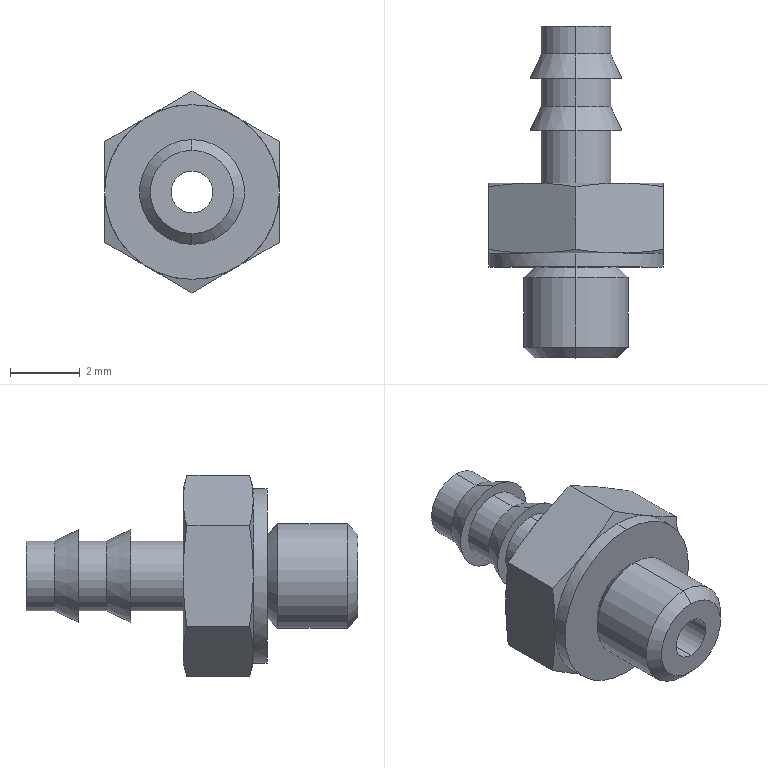Part | STEP file | M-3AU-3 | 1 solid | 44 faces | box 5 x 9.5 x 5.774 mm | volume 73.564 mm3 | cone 20 | cylinder 12 | plane 12 | commonest cylinder face diameters 2 x6 1.2 x2 3 x2 5 x2
STEP:
#1=CARTESIAN_POINT('',(0.,6.9,0.6));
#2=VERTEX_POINT('',#1);
#3=CARTESIAN_POINT('',(0.,6.9,-0.6));
#4=VERTEX_POINT('',#3);
#5=CARTESIAN_POINT('',(0.,6.9,0.));
#6=DIRECTION('',(0.,-1.,0.));
#7=DIRECTION('',(0.,0.,-1.));
#8=AXIS2_PLACEMENT_3D('',#5,#6,#7);
#9=CIRCLE('',#8,0.6);
#10=EDGE_CURVE('',#2,#4,#9,.T.);
#11=ORIENTED_EDGE('',*,*,#10,.F.);
#12=CARTESIAN_POINT('',(0.,-2.6,0.6));
#13=VERTEX_POINT('',#12);
#14=CARTESIAN_POINT('',(0.,2.15,0.6));
#15=DIRECTION('',(0.,-1.,0.));
#16=VECTOR('',#15,1000.);
#17=LINE('',#14,#16);
#18=EDGE_CURVE('',#2,#13,#17,.T.);
#19=ORIENTED_EDGE('',*,*,#18,.T.);
#20=CARTESIAN_POINT('',(0.,-2.6,-0.6));
#21=VERTEX_POINT('',#20);
#22=CARTESIAN_POINT('',(0.,-2.6,0.));
#23=DIRECTION('',(0.,1.,0.));
#24=DIRECTION('',(0.,0.,-1.));
#25=AXIS2_PLACEMENT_3D('',#22,#23,#24);
#26=CIRCLE('',#25,0.6);
#27=EDGE_CURVE('',#21,#13,#26,.T.);
#28=ORIENTED_EDGE('',*,*,#27,.F.);
#29=CARTESIAN_POINT('',(0.,2.15,-0.6));
#30=DIRECTION('',(0.,-1.,0.));
#31=VECTOR('',#30,1000.);
#32=LINE('',#29,#31);
#33=EDGE_CURVE('',#4,#21,#32,.T.);
#34=ORIENTED_EDGE('',*,*,#33,.F.);
#35=EDGE_LOOP('',(#11,#19,#28,#34));
#36=FACE_OUTER_BOUND('',#35,.T.);
#37=CARTESIAN_POINT('',(0.,2.15,0.));
#38=DIRECTION('',(0.,-1.,0.));
#39=DIRECTION('',(0.,0.,-1.));
#40=AXIS2_PLACEMENT_3D('',#37,#38,#39);
#41=CYLINDRICAL_SURFACE('',#40,0.6);
#42=ADVANCED_FACE('',(#36),#41,.F.);
#43=CARTESIAN_POINT('',(0.,-2.6,-1.193));
#44=VERTEX_POINT('',#43);
#45=CARTESIAN_POINT('',(0.,-2.6,1.193));
#46=VERTEX_POINT('',#45);
#47=CARTESIAN_POINT('',(0.,-2.6,0.));
#48=DIRECTION('',(0.,-1.,0.));
#49=DIRECTION('',(0.,0.,1.));
#50=AXIS2_PLACEMENT_3D('',#47,#48,#49);
#51=CIRCLE('',#50,1.193);
#52=EDGE_CURVE('',#44,#46,#51,.T.);
#53=ORIENTED_EDGE('',*,*,#52,.F.);
#54=CARTESIAN_POINT('',(0.,-2.294,-1.5));
#55=VERTEX_POINT('',#54);
#56=CARTESIAN_POINT('',(0.,-2.294,-1.5));
#57=DIRECTION('',(0.,0.7071,-0.7071));
#58=VECTOR('',#57,1000.);
#59=LINE('',#56,#58);
#60=EDGE_CURVE('',#44,#55,#59,.T.);
#61=ORIENTED_EDGE('',*,*,#60,.T.);
#62=CARTESIAN_POINT('',(0.,-2.294,1.5));
#63=VERTEX_POINT('',#62);
#64=CARTESIAN_POINT('',(0.,-2.294,0.));
#65=DIRECTION('',(0.,-1.,0.));
#66=DIRECTION('',(1.,0.,0.));
#67=AXIS2_PLACEMENT_3D('',#64,#65,#66);
#68=CIRCLE('',#67,1.5);
#69=EDGE_CURVE('',#55,#63,#68,.T.);
#70=ORIENTED_EDGE('',*,*,#69,.T.);
#71=CARTESIAN_POINT('',(0.,-2.294,1.5));
#72=DIRECTION('',(0.,0.7071,0.7071));
#73=VECTOR('',#72,1000.);
#74=LINE('',#71,#73);
#75=EDGE_CURVE('',#46,#63,#74,.T.);
#76=ORIENTED_EDGE('',*,*,#75,.F.);
#77=EDGE_LOOP('',(#53,#61,#70,#76));
#78=FACE_OUTER_BOUND('',#77,.T.);
#79=CARTESIAN_POINT('',(0.,-2.294,0.));
#80=DIRECTION('',(0.,1.,0.));
#81=DIRECTION('',(0.,0.,1.));
#82=AXIS2_PLACEMENT_3D('',#79,#80,#81);
#83=CONICAL_SURFACE('',#82,1.5,0.7854);
#84=ADVANCED_FACE('',(#78),#83,.T.);
#85=CARTESIAN_POINT('',(0.,6.9,1.));
#86=VERTEX_POINT('',#85);
#87=CARTESIAN_POINT('',(0.,6.9,-1.));
#88=VERTEX_POINT('',#87);
#89=CARTESIAN_POINT('',(0.,6.9,0.));
#90=DIRECTION('',(0.,1.,0.));
#91=DIRECTION('',(0.,0.,-1.));
#92=AXIS2_PLACEMENT_3D('',#89,#90,#91);
#93=CIRCLE('',#92,1.);
#94=EDGE_CURVE('',#86,#88,#93,.T.);
#95=ORIENTED_EDGE('',*,*,#94,.F.);
#96=CARTESIAN_POINT('',(0.,6.1,1.));
#97=VERTEX_POINT('',#96);
#98=CARTESIAN_POINT('',(0.,6.5,1.));
#99=DIRECTION('',(0.,-1.,0.));
#100=VECTOR('',#99,1000.);
#101=LINE('',#98,#100);
#102=EDGE_CURVE('',#86,#97,#101,.T.);
#103=ORIENTED_EDGE('',*,*,#102,.T.);
#104=CARTESIAN_POINT('',(0.,6.1,-1.));
#105=VERTEX_POINT('',#104);
#106=CARTESIAN_POINT('',(0.,6.1,0.));
#107=DIRECTION('',(0.,1.,0.));
#108=DIRECTION('',(0.,0.,-1.));
#109=AXIS2_PLACEMENT_3D('',#106,#107,#108);
#110=CIRCLE('',#109,1.);
#111=EDGE_CURVE('',#97,#105,#110,.T.);
#112=ORIENTED_EDGE('',*,*,#111,.T.);
#113=CARTESIAN_POINT('',(0.,6.5,-1.));
#114=DIRECTION('',(0.,-1.,0.));
#115=VECTOR('',#114,1000.);
#116=LINE('',#113,#115);
#117=EDGE_CURVE('',#88,#105,#116,.T.);
#118=ORIENTED_EDGE('',*,*,#117,.F.);
#119=EDGE_LOOP('',(#95,#103,#112,#118));
#120=FACE_OUTER_BOUND('',#119,.T.);
#121=CARTESIAN_POINT('',(0.,6.5,0.));
#122=DIRECTION('',(0.,-1.,0.));
#123=DIRECTION('',(0.,0.,-1.));
#124=AXIS2_PLACEMENT_3D('',#121,#122,#123);
#125=CYLINDRICAL_SURFACE('',#124,1.);
#126=ADVANCED_FACE('',(#120),#125,.T.);
#127=CARTESIAN_POINT('',(0.,-0.3065,-1.5));
#128=VERTEX_POINT('',#127);
#129=CARTESIAN_POINT('',(0.,-0.3065,1.5));
#130=VERTEX_POINT('',#129);
#131=CARTESIAN_POINT('',(0.,-0.3065,0.));
#132=DIRECTION('',(0.,-1.,0.));
#133=DIRECTION('',(0.,0.,-1.));
#134=AXIS2_PLACEMENT_3D('',#131,#132,#133);
#135=CIRCLE('',#134,1.5);
#136=EDGE_CURVE('',#128,#130,#135,.T.);
#137=ORIENTED_EDGE('',*,*,#136,.T.);
#138=CARTESIAN_POINT('',(0.,-1.3,1.5));
#139=DIRECTION('',(0.,-1.,0.));
#140=VECTOR('',#139,1000.);
#141=LINE('',#138,#140);
#142=EDGE_CURVE('',#130,#63,#141,.T.);
#143=ORIENTED_EDGE('',*,*,#142,.T.);
#144=ORIENTED_EDGE('',*,*,#69,.F.);
#145=CARTESIAN_POINT('',(0.,-1.3,-1.5));
#146=DIRECTION('',(0.,-1.,0.));
#147=VECTOR('',#146,1000.);
#148=LINE('',#145,#147);
#149=EDGE_CURVE('',#128,#55,#148,.T.);
#150=ORIENTED_EDGE('',*,*,#149,.F.);
#151=EDGE_LOOP('',(#137,#143,#144,#150));
#152=FACE_OUTER_BOUND('',#151,.T.);
#153=CARTESIAN_POINT('',(0.,-1.3,0.));
#154=DIRECTION('',(0.,-1.,0.));
#155=DIRECTION('',(0.,0.,-1.));
#156=AXIS2_PLACEMENT_3D('',#153,#154,#155);
#157=CYLINDRICAL_SURFACE('',#156,1.5);
#158=ADVANCED_FACE('',(#152),#157,.T.);
#159=ORIENTED_EDGE('',*,*,#111,.F.);
#160=CARTESIAN_POINT('',(0.,5.4,1.326));
#161=VERTEX_POINT('',#160);
#162=CARTESIAN_POINT('',(0.,5.4,1.326));
#163=DIRECTION('',(0.,-0.9063,0.4226));
#164=VECTOR('',#163,1000.);
#165=LINE('',#162,#164);
#166=EDGE_CURVE('',#97,#161,#165,.T.);
#167=ORIENTED_EDGE('',*,*,#166,.T.);
#168=CARTESIAN_POINT('',(0.,5.4,-1.326));
#169=VERTEX_POINT('',#168);
#170=CARTESIAN_POINT('',(0.,5.4,0.));
#171=DIRECTION('',(0.,1.,0.));
#172=DIRECTION('',(0.,0.,-1.));
#173=AXIS2_PLACEMENT_3D('',#170,#171,#172);
#174=CIRCLE('',#173,1.326);
#175=EDGE_CURVE('',#161,#169,#174,.T.);
#176=ORIENTED_EDGE('',*,*,#175,.T.);
#177=CARTESIAN_POINT('',(0.,5.4,-1.326));
#178=DIRECTION('',(0.,-0.9063,-0.4226));
#179=VECTOR('',#178,1000.);
#180=LINE('',#177,#179);
#181=EDGE_CURVE('',#105,#169,#180,.T.);
#182=ORIENTED_EDGE('',*,*,#181,.F.);
#183=EDGE_LOOP('',(#159,#167,#176,#182));
#184=FACE_OUTER_BOUND('',#183,.T.);
#185=CARTESIAN_POINT('',(0.,5.4,0.));
#186=DIRECTION('',(0.,-1.,0.));
#187=DIRECTION('',(0.,0.,-1.));
#188=AXIS2_PLACEMENT_3D('',#185,#186,#187);
#189=CONICAL_SURFACE('',#188,1.326,0.4363);
#190=ADVANCED_FACE('',(#184),#189,.T.);
#191=CARTESIAN_POINT('',(0.,0.,-1.193));
#192=VERTEX_POINT('',#191);
#193=CARTESIAN_POINT('',(0.,0.,1.193));
#194=VERTEX_POINT('',#193);
#195=CARTESIAN_POINT('',(0.,0.,0.));
#196=DIRECTION('',(0.,-1.,0.));
#197=DIRECTION('',(0.,0.,-1.));
#198=AXIS2_PLACEMENT_3D('',#195,#196,#197);
#199=CIRCLE('',#198,1.193);
#200=EDGE_CURVE('',#192,#194,#199,.T.);
#201=ORIENTED_EDGE('',*,*,#200,.T.);
#202=CARTESIAN_POINT('',(0.,-0.3065,1.5));
#203=DIRECTION('',(0.,-0.7071,0.7071));
#204=VECTOR('',#203,1000.);
#205=LINE('',#202,#204);
#206=EDGE_CURVE('',#194,#130,#205,.T.);
#207=ORIENTED_EDGE('',*,*,#206,.T.);
#208=ORIENTED_EDGE('',*,*,#136,.F.);
#209=CARTESIAN_POINT('',(0.,-0.3065,-1.5));
#210=DIRECTION('',(0.,-0.7071,-0.7071));
#211=VECTOR('',#210,1000.);
#212=LINE('',#209,#211);
#213=EDGE_CURVE('',#192,#128,#212,.T.);
#214=ORIENTED_EDGE('',*,*,#213,.F.);
#215=EDGE_LOOP('',(#201,#207,#208,#214));
#216=FACE_OUTER_BOUND('',#215,.T.);
#217=CARTESIAN_POINT('',(0.,-0.3065,0.));
#218=DIRECTION('',(0.,-1.,0.));
#219=DIRECTION('',(0.,0.,-1.));
#220=AXIS2_PLACEMENT_3D('',#217,#218,#219);
#221=CONICAL_SURFACE('',#220,1.5,0.7854);
#222=ADVANCED_FACE('',(#216),#221,.T.);
#223=CARTESIAN_POINT('',(0.,5.4,1.));
#224=VERTEX_POINT('',#223);
#225=CARTESIAN_POINT('',(0.,5.4,-1.));
#226=VERTEX_POINT('',#225);
#227=CARTESIAN_POINT('',(0.,5.4,0.));
#228=DIRECTION('',(0.,1.,0.));
#229=DIRECTION('',(0.,0.,-1.));
#230=AXIS2_PLACEMENT_3D('',#227,#228,#229);
#231=CIRCLE('',#230,1.);
#232=EDGE_CURVE('',#224,#226,#231,.T.);
#233=ORIENTED_EDGE('',*,*,#232,.F.);
#234=CARTESIAN_POINT('',(0.,4.6,1.));
#235=VERTEX_POINT('',#234);
#236=CARTESIAN_POINT('',(0.,5.,1.));
#237=DIRECTION('',(0.,-1.,0.));
#238=VECTOR('',#237,1000.);
#239=LINE('',#236,#238);
#240=EDGE_CURVE('',#224,#235,#239,.T.);
#241=ORIENTED_EDGE('',*,*,#240,.T.);
#242=CARTESIAN_POINT('',(0.,4.6,-1.));
#243=VERTEX_POINT('',#242);
#244=CARTESIAN_POINT('',(0.,4.6,0.));
#245=DIRECTION('',(0.,1.,0.));
#246=DIRECTION('',(0.,0.,-1.));
#247=AXIS2_PLACEMENT_3D('',#244,#245,#246);
#248=CIRCLE('',#247,1.);
#249=EDGE_CURVE('',#235,#243,#248,.T.);
#250=ORIENTED_EDGE('',*,*,#249,.T.);
#251=CARTESIAN_POINT('',(0.,5.,-1.));
#252=DIRECTION('',(0.,-1.,0.));
#253=VECTOR('',#252,1000.);
#254=LINE('',#251,#253);
#255=EDGE_CURVE('',#226,#243,#254,.T.);
#256=ORIENTED_EDGE('',*,*,#255,.F.);
#257=EDGE_LOOP('',(#233,#241,#250,#256));
#258=FACE_OUTER_BOUND('',#257,.T.);
#259=CARTESIAN_POINT('',(0.,5.,0.));
#260=DIRECTION('',(0.,-1.,0.));
#261=DIRECTION('',(0.,0.,-1.));
#262=AXIS2_PLACEMENT_3D('',#259,#260,#261);
#263=CYLINDRICAL_SURFACE('',#262,1.);
#264=ADVANCED_FACE('',(#258),#263,.T.);
#265=CARTESIAN_POINT('',(1.25,0.4,2.165));
#266=VERTEX_POINT('',#265);
#267=CARTESIAN_POINT('',(0.,0.4,2.5));
#268=VERTEX_POINT('',#267);
#269=CARTESIAN_POINT('',(0.,0.4,0.));
#270=DIRECTION('',(0.,-1.,0.));
#271=DIRECTION('',(0.,0.,-1.));
#272=AXIS2_PLACEMENT_3D('',#269,#270,#271);
#273=CIRCLE('',#272,2.5);
#274=EDGE_CURVE('',#266,#268,#273,.T.);
#275=ORIENTED_EDGE('',*,*,#274,.T.);
#276=CARTESIAN_POINT('',(0.,0.,2.5));
#277=VERTEX_POINT('',#276);
#278=CARTESIAN_POINT('',(0.,0.2,2.5));
#279=DIRECTION('',(0.,-1.,0.));
#280=VECTOR('',#279,1000.);
#281=LINE('',#278,#280);
#282=EDGE_CURVE('',#268,#277,#281,.T.);
#283=ORIENTED_EDGE('',*,*,#282,.T.);
#284=CARTESIAN_POINT('',(0.,0.,-2.5));
#285=VERTEX_POINT('',#284);
#286=CARTESIAN_POINT('',(0.,0.,0.));
#287=DIRECTION('',(0.,-1.,0.));
#288=DIRECTION('',(0.,0.,-1.));
#289=AXIS2_PLACEMENT_3D('',#286,#287,#288);
#290=CIRCLE('',#289,2.5);
#291=EDGE_CURVE('',#285,#277,#290,.T.);
#292=ORIENTED_EDGE('',*,*,#291,.F.);
#293=CARTESIAN_POINT('',(0.,0.4,-2.5));
#294=VERTEX_POINT('',#293);
#295=CARTESIAN_POINT('',(0.,0.2,-2.5));
#296=DIRECTION('',(0.,-1.,0.));
#297=VECTOR('',#296,1000.);
#298=LINE('',#295,#297);
#299=EDGE_CURVE('',#294,#285,#298,.T.);
#300=ORIENTED_EDGE('',*,*,#299,.F.);
#301=CARTESIAN_POINT('',(1.25,0.4,-2.165));
#302=VERTEX_POINT('',#301);
#303=CARTESIAN_POINT('',(0.,0.4,0.));
#304=DIRECTION('',(0.,-1.,0.));
#305=DIRECTION('',(0.,0.,-1.));
#306=AXIS2_PLACEMENT_3D('',#303,#304,#305);
#307=CIRCLE('',#306,2.5);
#308=EDGE_CURVE('',#294,#302,#307,.T.);
#309=ORIENTED_EDGE('',*,*,#308,.T.);
#310=CARTESIAN_POINT('',(2.5,0.4,0.));
#311=VERTEX_POINT('',#310);
#312=CARTESIAN_POINT('',(0.,0.4,0.));
#313=DIRECTION('',(0.,-1.,0.));
#314=DIRECTION('',(0.,0.,-1.));
#315=AXIS2_PLACEMENT_3D('',#312,#313,#314);
#316=CIRCLE('',#315,2.5);
#317=EDGE_CURVE('',#302,#311,#316,.T.);
#318=ORIENTED_EDGE('',*,*,#317,.T.);
#319=CARTESIAN_POINT('',(0.,0.4,0.));
#320=DIRECTION('',(0.,-1.,0.));
#321=DIRECTION('',(0.,0.,-1.));
#322=AXIS2_PLACEMENT_3D('',#319,#320,#321);
#323=CIRCLE('',#322,2.5);
#324=EDGE_CURVE('',#311,#266,#323,.T.);
#325=ORIENTED_EDGE('',*,*,#324,.T.);
#326=EDGE_LOOP('',(#275,#283,#292,#300,#309,#318,#325));
#327=FACE_OUTER_BOUND('',#326,.T.);
#328=CARTESIAN_POINT('',(0.,0.2,0.));
#329=DIRECTION('',(0.,-1.,0.));
#330=DIRECTION('',(0.,0.,-1.));
#331=AXIS2_PLACEMENT_3D('',#328,#329,#330);
#332=CYLINDRICAL_SURFACE('',#331,2.5);
#333=ADVANCED_FACE('',(#327),#332,.T.);
#334=ORIENTED_EDGE('',*,*,#249,.F.);
#335=CARTESIAN_POINT('',(0.,3.9,1.326));
#336=VERTEX_POINT('',#335);
#337=CARTESIAN_POINT('',(0.,3.9,1.326));
#338=DIRECTION('',(0.,-0.9063,0.4226));
#339=VECTOR('',#338,1000.);
#340=LINE('',#337,#339);
#341=EDGE_CURVE('',#235,#336,#340,.T.);
#342=ORIENTED_EDGE('',*,*,#341,.T.);
#343=CARTESIAN_POINT('',(0.,3.9,-1.326));
#344=VERTEX_POINT('',#343);
#345=CARTESIAN_POINT('',(0.,3.9,0.));
#346=DIRECTION('',(0.,1.,0.));
#347=DIRECTION('',(0.,0.,-1.));
#348=AXIS2_PLACEMENT_3D('',#345,#346,#347);
#349=CIRCLE('',#348,1.326);
#350=EDGE_CURVE('',#336,#344,#349,.T.);
#351=ORIENTED_EDGE('',*,*,#350,.T.);
#352=CARTESIAN_POINT('',(0.,3.9,-1.326));
#353=DIRECTION('',(0.,-0.9063,-0.4226));
#354=VECTOR('',#353,1000.);
#355=LINE('',#352,#354);
#356=EDGE_CURVE('',#243,#344,#355,.T.);
#357=ORIENTED_EDGE('',*,*,#356,.F.);
#358=EDGE_LOOP('',(#334,#342,#351,#357));
#359=FACE_OUTER_BOUND('',#358,.T.);
#360=CARTESIAN_POINT('',(0.,3.9,0.));
#361=DIRECTION('',(0.,-1.,0.));
#362=DIRECTION('',(0.,0.,-1.));
#363=AXIS2_PLACEMENT_3D('',#360,#361,#362);
#364=CONICAL_SURFACE('',#363,1.326,0.4363);
#365=ADVANCED_FACE('',(#359),#364,.T.);
#366=CARTESIAN_POINT('',(0.,3.9,1.));
#367=VERTEX_POINT('',#366);
#368=CARTESIAN_POINT('',(0.,3.9,-1.));
#369=VERTEX_POINT('',#368);
#370=CARTESIAN_POINT('',(0.,3.9,0.));
#371=DIRECTION('',(0.,1.,0.));
#372=DIRECTION('',(0.,0.,-1.));
#373=AXIS2_PLACEMENT_3D('',#370,#371,#372);
#374=CIRCLE('',#373,1.);
#375=EDGE_CURVE('',#367,#369,#374,.T.);
#376=ORIENTED_EDGE('',*,*,#375,.F.);
#377=CARTESIAN_POINT('',(0.,2.4,1.));
#378=VERTEX_POINT('',#377);
#379=CARTESIAN_POINT('',(0.,3.15,1.));
#380=DIRECTION('',(0.,-1.,0.));
#381=VECTOR('',#380,1000.);
#382=LINE('',#379,#381);
#383=EDGE_CURVE('',#367,#378,#382,.T.);
#384=ORIENTED_EDGE('',*,*,#383,.T.);
#385=CARTESIAN_POINT('',(0.,2.4,-1.));
#386=VERTEX_POINT('',#385);
#387=CARTESIAN_POINT('',(0.,2.4,0.));
#388=DIRECTION('',(0.,1.,0.));
#389=DIRECTION('',(0.,0.,-1.));
#390=AXIS2_PLACEMENT_3D('',#387,#388,#389);
#391=CIRCLE('',#390,1.);
#392=EDGE_CURVE('',#378,#386,#391,.T.);
#393=ORIENTED_EDGE('',*,*,#392,.T.);
#394=CARTESIAN_POINT('',(0.,3.15,-1.));
#395=DIRECTION('',(0.,-1.,0.));
#396=VECTOR('',#395,1000.);
#397=LINE('',#394,#396);
#398=EDGE_CURVE('',#369,#386,#397,.T.);
#399=ORIENTED_EDGE('',*,*,#398,.F.);
#400=EDGE_LOOP('',(#376,#384,#393,#399));
#401=FACE_OUTER_BOUND('',#400,.T.);
#402=CARTESIAN_POINT('',(0.,3.15,0.));
#403=DIRECTION('',(0.,-1.,0.));
#404=DIRECTION('',(0.,0.,-1.));
#405=AXIS2_PLACEMENT_3D('',#402,#403,#404);
#406=CYLINDRICAL_SURFACE('',#405,1.);
#407=ADVANCED_FACE('',(#401),#406,.T.);
#408=ORIENTED_EDGE('',*,*,#18,.F.);
#409=CARTESIAN_POINT('',(0.,6.9,0.));
#410=DIRECTION('',(0.,-1.,0.));
#411=DIRECTION('',(0.,0.,-1.));
#412=AXIS2_PLACEMENT_3D('',#409,#410,#411);
#413=CIRCLE('',#412,0.6);
#414=EDGE_CURVE('',#4,#2,#413,.T.);
#415=ORIENTED_EDGE('',*,*,#414,.F.);
#416=ORIENTED_EDGE('',*,*,#33,.T.);
#417=CARTESIAN_POINT('',(0.,-2.6,0.));
#418=DIRECTION('',(0.,1.,0.));
#419=DIRECTION('',(0.,0.,-1.));
#420=AXIS2_PLACEMENT_3D('',#417,#418,#419);
#421=CIRCLE('',#420,0.6);
#422=EDGE_CURVE('',#13,#21,#421,.T.);
#423=ORIENTED_EDGE('',*,*,#422,.F.);
#424=EDGE_LOOP('',(#408,#415,#416,#423));
#425=FACE_OUTER_BOUND('',#424,.T.);
#426=CARTESIAN_POINT('',(0.,2.15,0.));
#427=DIRECTION('',(0.,-1.,0.));
#428=DIRECTION('',(0.,0.,-1.));
#429=AXIS2_PLACEMENT_3D('',#426,#427,#428);
#430=CYLINDRICAL_SURFACE('',#429,0.6);
#431=ADVANCED_FACE('',(#425),#430,.F.);
#432=ORIENTED_EDGE('',*,*,#27,.T.);
#433=ORIENTED_EDGE('',*,*,#422,.T.);
#434=EDGE_LOOP('',(#432,#433));
#435=FACE_BOUND('',#434,.T.);
#436=CARTESIAN_POINT('',(0.,-2.6,0.));
#437=DIRECTION('',(0.,-1.,0.));
#438=DIRECTION('',(0.,0.,1.));
#439=AXIS2_PLACEMENT_3D('',#436,#437,#438);
#440=CIRCLE('',#439,1.193);
#441=EDGE_CURVE('',#46,#44,#440,.T.);
#442=ORIENTED_EDGE('',*,*,#441,.T.);
#443=ORIENTED_EDGE('',*,*,#52,.T.);
#444=EDGE_LOOP('',(#442,#443));
#445=FACE_OUTER_BOUND('',#444,.T.);
#446=CARTESIAN_POINT('',(0.8967,-2.6,0.));
#447=DIRECTION('',(0.,-1.,0.));
#448=DIRECTION('',(1.,0.,0.));
#449=AXIS2_PLACEMENT_3D('',#446,#447,#448);
#450=PLANE('',#449);
#451=ADVANCED_FACE('',(#435,#445),#450,.T.);
#452=CARTESIAN_POINT('',(0.,6.9,0.));
#453=DIRECTION('',(0.,1.,0.));
#454=DIRECTION('',(0.,0.,-1.));
#455=AXIS2_PLACEMENT_3D('',#452,#453,#454);
#456=CIRCLE('',#455,1.);
#457=EDGE_CURVE('',#88,#86,#456,.T.);
#458=ORIENTED_EDGE('',*,*,#457,.T.);
#459=ORIENTED_EDGE('',*,*,#94,.T.);
#460=EDGE_LOOP('',(#458,#459));
#461=FACE_OUTER_BOUND('',#460,.T.);
#462=ORIENTED_EDGE('',*,*,#414,.T.);
#463=ORIENTED_EDGE('',*,*,#10,.T.);
#464=EDGE_LOOP('',(#462,#463));
#465=FACE_BOUND('',#464,.T.);
#466=CARTESIAN_POINT('',(0.8,6.9,0.));
#467=DIRECTION('',(0.,1.,0.));
#468=DIRECTION('',(0.,0.,1.));
#469=AXIS2_PLACEMENT_3D('',#466,#467,#468);
#470=PLANE('',#469);
#471=ADVANCED_FACE('',(#461,#465),#470,.T.);
#472=ORIENTED_EDGE('',*,*,#60,.F.);
#473=ORIENTED_EDGE('',*,*,#441,.F.);
#474=ORIENTED_EDGE('',*,*,#75,.T.);
#475=CARTESIAN_POINT('',(0.,-2.294,0.));
#476=DIRECTION('',(0.,-1.,0.));
#477=DIRECTION('',(1.,0.,0.));
#478=AXIS2_PLACEMENT_3D('',#475,#476,#477);
#479=CIRCLE('',#478,1.5);
#480=EDGE_CURVE('',#63,#55,#479,.T.);
#481=ORIENTED_EDGE('',*,*,#480,.T.);
#482=EDGE_LOOP('',(#472,#473,#474,#481));
#483=FACE_OUTER_BOUND('',#482,.T.);
#484=CARTESIAN_POINT('',(0.,-2.294,0.));
#485=DIRECTION('',(0.,1.,0.));
#486=DIRECTION('',(0.,0.,1.));
#487=AXIS2_PLACEMENT_3D('',#484,#485,#486);
#488=CONICAL_SURFACE('',#487,1.5,0.7854);
#489=ADVANCED_FACE('',(#483),#488,.T.);
#490=ORIENTED_EDGE('',*,*,#102,.F.);
#491=ORIENTED_EDGE('',*,*,#457,.F.);
#492=ORIENTED_EDGE('',*,*,#117,.T.);
#493=CARTESIAN_POINT('',(0.,6.1,0.));
#494=DIRECTION('',(0.,1.,0.));
#495=DIRECTION('',(0.,0.,-1.));
#496=AXIS2_PLACEMENT_3D('',#493,#494,#495);
#497=CIRCLE('',#496,1.);
#498=EDGE_CURVE('',#105,#97,#497,.T.);
#499=ORIENTED_EDGE('',*,*,#498,.T.);
#500=EDGE_LOOP('',(#490,#491,#492,#499));
#501=FACE_OUTER_BOUND('',#500,.T.);
#502=CARTESIAN_POINT('',(0.,6.5,0.));
#503=DIRECTION('',(0.,-1.,0.));
#504=DIRECTION('',(0.,0.,-1.));
#505=AXIS2_PLACEMENT_3D('',#502,#503,#504);
#506=CYLINDRICAL_SURFACE('',#505,1.);
#507=ADVANCED_FACE('',(#501),#506,.T.);
#508=ORIENTED_EDGE('',*,*,#142,.F.);
#509=CARTESIAN_POINT('',(0.,-0.3065,0.));
#510=DIRECTION('',(0.,-1.,0.));
#511=DIRECTION('',(0.,0.,-1.));
#512=AXIS2_PLACEMENT_3D('',#509,#510,#511);
#513=CIRCLE('',#512,1.5);
#514=EDGE_CURVE('',#130,#128,#513,.T.);
#515=ORIENTED_EDGE('',*,*,#514,.T.);
#516=ORIENTED_EDGE('',*,*,#149,.T.);
#517=ORIENTED_EDGE('',*,*,#480,.F.);
#518=EDGE_LOOP('',(#508,#515,#516,#517));
#519=FACE_OUTER_BOUND('',#518,.T.);
#520=CARTESIAN_POINT('',(0.,-1.3,0.));
#521=DIRECTION('',(0.,-1.,0.));
#522=DIRECTION('',(0.,0.,-1.));
#523=AXIS2_PLACEMENT_3D('',#520,#521,#522);
#524=CYLINDRICAL_SURFACE('',#523,1.5);
#525=ADVANCED_FACE('',(#519),#524,.T.);
#526=ORIENTED_EDGE('',*,*,#166,.F.);
#527=ORIENTED_EDGE('',*,*,#498,.F.);
#528=ORIENTED_EDGE('',*,*,#181,.T.);
#529=CARTESIAN_POINT('',(0.,5.4,0.));
#530=DIRECTION('',(0.,1.,0.));
#531=DIRECTION('',(0.,0.,-1.));
#532=AXIS2_PLACEMENT_3D('',#529,#530,#531);
#533=CIRCLE('',#532,1.326);
#534=EDGE_CURVE('',#169,#161,#533,.T.);
#535=ORIENTED_EDGE('',*,*,#534,.T.);
#536=EDGE_LOOP('',(#526,#527,#528,#535));
#537=FACE_OUTER_BOUND('',#536,.T.);
#538=CARTESIAN_POINT('',(0.,5.4,0.));
#539=DIRECTION('',(0.,-1.,0.));
#540=DIRECTION('',(0.,0.,-1.));
#541=AXIS2_PLACEMENT_3D('',#538,#539,#540);
#542=CONICAL_SURFACE('',#541,1.326,0.4363);
#543=ADVANCED_FACE('',(#537),#542,.T.);
#544=ORIENTED_EDGE('',*,*,#206,.F.);
#545=CARTESIAN_POINT('',(0.,0.,0.));
#546=DIRECTION('',(0.,-1.,0.));
#547=DIRECTION('',(0.,0.,-1.));
#548=AXIS2_PLACEMENT_3D('',#545,#546,#547);
#549=CIRCLE('',#548,1.193);
#550=EDGE_CURVE('',#194,#192,#549,.T.);
#551=ORIENTED_EDGE('',*,*,#550,.T.);
#552=ORIENTED_EDGE('',*,*,#213,.T.);
#553=ORIENTED_EDGE('',*,*,#514,.F.);
#554=EDGE_LOOP('',(#544,#551,#552,#553));
#555=FACE_OUTER_BOUND('',#554,.T.);
#556=CARTESIAN_POINT('',(0.,-0.3065,0.));
#557=DIRECTION('',(0.,-1.,0.));
#558=DIRECTION('',(0.,0.,-1.));
#559=AXIS2_PLACEMENT_3D('',#556,#557,#558);
#560=CONICAL_SURFACE('',#559,1.5,0.7854);
#561=ADVANCED_FACE('',(#555),#560,.T.);
#562=CARTESIAN_POINT('',(0.,5.4,0.));
#563=DIRECTION('',(0.,1.,0.));
#564=DIRECTION('',(0.,0.,-1.));
#565=AXIS2_PLACEMENT_3D('',#562,#563,#564);
#566=CIRCLE('',#565,1.);
#567=EDGE_CURVE('',#226,#224,#566,.T.);
#568=ORIENTED_EDGE('',*,*,#567,.T.);
#569=ORIENTED_EDGE('',*,*,#232,.T.);
#570=EDGE_LOOP('',(#568,#569));
#571=FACE_BOUND('',#570,.T.);
#572=ORIENTED_EDGE('',*,*,#534,.F.);
#573=ORIENTED_EDGE('',*,*,#175,.F.);
#574=EDGE_LOOP('',(#572,#573));
#575=FACE_OUTER_BOUND('',#574,.T.);
#576=CARTESIAN_POINT('',(1.163,5.4,0.));
#577=DIRECTION('',(0.,-1.,0.));
#578=DIRECTION('',(0.,0.,-1.));
#579=AXIS2_PLACEMENT_3D('',#576,#577,#578);
#580=PLANE('',#579);
#581=ADVANCED_FACE('',(#571,#575),#580,.T.);
#582=ORIENTED_EDGE('',*,*,#200,.F.);
#583=ORIENTED_EDGE('',*,*,#550,.F.);
#584=EDGE_LOOP('',(#582,#583));
#585=FACE_BOUND('',#584,.T.);
#586=ORIENTED_EDGE('',*,*,#291,.T.);
#587=CARTESIAN_POINT('',(0.,0.,0.));
#588=DIRECTION('',(0.,-1.,0.));
#589=DIRECTION('',(0.,0.,-1.));
#590=AXIS2_PLACEMENT_3D('',#587,#588,#589);
#591=CIRCLE('',#590,2.5);
#592=EDGE_CURVE('',#277,#285,#591,.T.);
#593=ORIENTED_EDGE('',*,*,#592,.T.);
#594=EDGE_LOOP('',(#586,#593));
#595=FACE_OUTER_BOUND('',#594,.T.);
#596=CARTESIAN_POINT('',(1.847,0.,0.));
#597=DIRECTION('',(0.,-1.,0.));
#598=DIRECTION('',(0.,0.,-1.));
#599=AXIS2_PLACEMENT_3D('',#596,#597,#598);
#600=PLANE('',#599);
#601=ADVANCED_FACE('',(#585,#595),#600,.T.);
#602=ORIENTED_EDGE('',*,*,#240,.F.);
#603=ORIENTED_EDGE('',*,*,#567,.F.);
#604=ORIENTED_EDGE('',*,*,#255,.T.);
#605=CARTESIAN_POINT('',(0.,4.6,0.));
#606=DIRECTION('',(0.,1.,0.));
#607=DIRECTION('',(0.,0.,-1.));
#608=AXIS2_PLACEMENT_3D('',#605,#606,#607);
#609=CIRCLE('',#608,1.);
#610=EDGE_CURVE('',#243,#235,#609,.T.);
#611=ORIENTED_EDGE('',*,*,#610,.T.);
#612=EDGE_LOOP('',(#602,#603,#604,#611));
#613=FACE_OUTER_BOUND('',#612,.T.);
#614=CARTESIAN_POINT('',(0.,5.,0.));
#615=DIRECTION('',(0.,-1.,0.));
#616=DIRECTION('',(0.,0.,-1.));
#617=AXIS2_PLACEMENT_3D('',#614,#615,#616);
#618=CYLINDRICAL_SURFACE('',#617,1.);
#619=ADVANCED_FACE('',(#613),#618,.T.);
#620=ORIENTED_EDGE('',*,*,#282,.F.);
#621=CARTESIAN_POINT('',(-1.25,0.4,2.165));
#622=VERTEX_POINT('',#621);
#623=CARTESIAN_POINT('',(0.,0.4,0.));
#624=DIRECTION('',(0.,-1.,0.));
#625=DIRECTION('',(0.,0.,-1.));
#626=AXIS2_PLACEMENT_3D('',#623,#624,#625);
#627=CIRCLE('',#626,2.5);
#628=EDGE_CURVE('',#268,#622,#627,.T.);
#629=ORIENTED_EDGE('',*,*,#628,.T.);
#630=CARTESIAN_POINT('',(-2.5,0.4,0.));
#631=VERTEX_POINT('',#630);
#632=CARTESIAN_POINT('',(0.,0.4,0.));
#633=DIRECTION('',(0.,-1.,0.));
#634=DIRECTION('',(0.,0.,-1.));
#635=AXIS2_PLACEMENT_3D('',#632,#633,#634);
#636=CIRCLE('',#635,2.5);
#637=EDGE_CURVE('',#622,#631,#636,.T.);
#638=ORIENTED_EDGE('',*,*,#637,.T.);
#639=CARTESIAN_POINT('',(-1.25,0.4,-2.165));
#640=VERTEX_POINT('',#639);
#641=CARTESIAN_POINT('',(0.,0.4,0.));
#642=DIRECTION('',(0.,-1.,0.));
#643=DIRECTION('',(0.,0.,-1.));
#644=AXIS2_PLACEMENT_3D('',#641,#642,#643);
#645=CIRCLE('',#644,2.5);
#646=EDGE_CURVE('',#631,#640,#645,.T.);
#647=ORIENTED_EDGE('',*,*,#646,.T.);
#648=CARTESIAN_POINT('',(0.,0.4,0.));
#649=DIRECTION('',(0.,-1.,0.));
#650=DIRECTION('',(0.,0.,-1.));
#651=AXIS2_PLACEMENT_3D('',#648,#649,#650);
#652=CIRCLE('',#651,2.5);
#653=EDGE_CURVE('',#640,#294,#652,.T.);
#654=ORIENTED_EDGE('',*,*,#653,.T.);
#655=ORIENTED_EDGE('',*,*,#299,.T.);
#656=ORIENTED_EDGE('',*,*,#592,.F.);
#657=EDGE_LOOP('',(#620,#629,#638,#647,#654,#655,#656));
#658=FACE_OUTER_BOUND('',#657,.T.);
#659=CARTESIAN_POINT('',(0.,0.2,0.));
#660=DIRECTION('',(0.,-1.,0.));
#661=DIRECTION('',(0.,0.,-1.));
#662=AXIS2_PLACEMENT_3D('',#659,#660,#661);
#663=CYLINDRICAL_SURFACE('',#662,2.5);
#664=ADVANCED_FACE('',(#658),#663,.T.);
#665=ORIENTED_EDGE('',*,*,#341,.F.);
#666=ORIENTED_EDGE('',*,*,#610,.F.);
#667=ORIENTED_EDGE('',*,*,#356,.T.);
#668=CARTESIAN_POINT('',(0.,3.9,0.));
#669=DIRECTION('',(0.,1.,0.));
#670=DIRECTION('',(0.,0.,-1.));
#671=AXIS2_PLACEMENT_3D('',#668,#669,#670);
#672=CIRCLE('',#671,1.326);
#673=EDGE_CURVE('',#344,#336,#672,.T.);
#674=ORIENTED_EDGE('',*,*,#673,.T.);
#675=EDGE_LOOP('',(#665,#666,#667,#674));
#676=FACE_OUTER_BOUND('',#675,.T.);
#677=CARTESIAN_POINT('',(0.,3.9,0.));
#678=DIRECTION('',(0.,-1.,0.));
#679=DIRECTION('',(0.,0.,-1.));
#680=AXIS2_PLACEMENT_3D('',#677,#678,#679);
#681=CONICAL_SURFACE('',#680,1.326,0.4363);
#682=ADVANCED_FACE('',(#676),#681,.T.);
#683=ORIENTED_EDGE('',*,*,#317,.F.);
#684=CARTESIAN_POINT('',(2.5,0.5036,-1.443));
#685=VERTEX_POINT('',#684);
#686=CARTESIAN_POINT('',(1.25,0.4,-2.165));
#687=CARTESIAN_POINT('',(1.669,0.4,-1.923));
#688=CARTESIAN_POINT('',(2.085,0.4395,-1.683));
#689=CARTESIAN_POINT('',(2.5,0.5036,-1.443));
#690=B_SPLINE_CURVE_WITH_KNOTS('',3,(#686,#687,#688,#689),.UNSPECIFIED.,.F.,.F.,(4,4),(0.,0.001447),.UNSPECIFIED.);
#691=EDGE_CURVE('',#302,#685,#690,.T.);
#692=ORIENTED_EDGE('',*,*,#691,.T.);
#693=CARTESIAN_POINT('',(2.5,0.5036,-1.443));
#694=CARTESIAN_POINT('',(2.5,0.4395,-0.9644));
#695=CARTESIAN_POINT('',(2.5,0.4,-0.4836));
#696=CARTESIAN_POINT('',(2.5,0.4,0.));
#697=B_SPLINE_CURVE_WITH_KNOTS('',3,(#693,#694,#695,#696),.UNSPECIFIED.,.F.,.F.,(4,4),(0.,0.001447),.UNSPECIFIED.);
#698=EDGE_CURVE('',#685,#311,#697,.T.);
#699=ORIENTED_EDGE('',*,*,#698,.T.);
#700=EDGE_LOOP('',(#683,#692,#699));
#701=FACE_OUTER_BOUND('',#700,.T.);
#702=CARTESIAN_POINT('',(0.,0.5043,0.));
#703=DIRECTION('',(0.,1.,0.));
#704=DIRECTION('',(-1.,0.,0.));
#705=AXIS2_PLACEMENT_3D('',#702,#703,#704);
#706=CONICAL_SURFACE('',#705,2.889,1.309);
#707=ADVANCED_FACE('',(#701),#706,.T.);
#708=ORIENTED_EDGE('',*,*,#653,.F.);
#709=CARTESIAN_POINT('',(0.00000002,0.5036,-2.887));
#710=VERTEX_POINT('',#709);
#711=CARTESIAN_POINT('',(-1.25,0.4,-2.165));
#712=CARTESIAN_POINT('',(-0.8312,0.4,-2.407));
#713=CARTESIAN_POINT('',(-0.4148,0.4395,-2.647));
#714=CARTESIAN_POINT('',(0.00000002,0.5036,-2.887));
#715=B_SPLINE_CURVE_WITH_KNOTS('',3,(#711,#712,#713,#714),.UNSPECIFIED.,.F.,.F.,(4,4),(0.,0.001447),.UNSPECIFIED.);
#716=EDGE_CURVE('',#640,#710,#715,.T.);
#717=ORIENTED_EDGE('',*,*,#716,.T.);
#718=CARTESIAN_POINT('',(0.00000002,0.5036,-2.887));
#719=CARTESIAN_POINT('',(0.4148,0.4395,-2.647));
#720=CARTESIAN_POINT('',(0.8312,0.4,-2.407));
#721=CARTESIAN_POINT('',(1.25,0.4,-2.165));
#722=B_SPLINE_CURVE_WITH_KNOTS('',3,(#718,#719,#720,#721),.UNSPECIFIED.,.F.,.F.,(4,4),(0.,0.001447),.UNSPECIFIED.);
#723=EDGE_CURVE('',#710,#302,#722,.T.);
#724=ORIENTED_EDGE('',*,*,#723,.T.);
#725=ORIENTED_EDGE('',*,*,#308,.F.);
#726=EDGE_LOOP('',(#708,#717,#724,#725));
#727=FACE_OUTER_BOUND('',#726,.T.);
#728=CARTESIAN_POINT('',(0.,0.5043,0.));
#729=DIRECTION('',(0.,1.,0.));
#730=DIRECTION('',(-1.,0.,0.));
#731=AXIS2_PLACEMENT_3D('',#728,#729,#730);
#732=CONICAL_SURFACE('',#731,2.889,1.309);
#733=ADVANCED_FACE('',(#727),#732,.T.);
#734=CARTESIAN_POINT('',(-2.5,0.5036,-1.443));
#735=VERTEX_POINT('',#734);
#736=CARTESIAN_POINT('',(-2.5,0.5036,-1.443));
#737=CARTESIAN_POINT('',(-2.085,0.4395,-1.683));
#738=CARTESIAN_POINT('',(-1.669,0.4,-1.923));
#739=CARTESIAN_POINT('',(-1.25,0.4,-2.165));
#740=B_SPLINE_CURVE_WITH_KNOTS('',3,(#736,#737,#738,#739),.UNSPECIFIED.,.F.,.F.,(4,4),(0.,0.001447),.UNSPECIFIED.);
#741=EDGE_CURVE('',#735,#640,#740,.T.);
#742=ORIENTED_EDGE('',*,*,#741,.T.);
#743=ORIENTED_EDGE('',*,*,#646,.F.);
#744=CARTESIAN_POINT('',(-2.5,0.4,0.));
#745=CARTESIAN_POINT('',(-2.5,0.4,-0.4836));
#746=CARTESIAN_POINT('',(-2.5,0.4395,-0.9644));
#747=CARTESIAN_POINT('',(-2.5,0.5036,-1.443));
#748=B_SPLINE_CURVE_WITH_KNOTS('',3,(#744,#745,#746,#747),.UNSPECIFIED.,.F.,.F.,(4,4),(0.,0.001447),.UNSPECIFIED.);
#749=EDGE_CURVE('',#631,#735,#748,.T.);
#750=ORIENTED_EDGE('',*,*,#749,.T.);
#751=EDGE_LOOP('',(#742,#743,#750));
#752=FACE_OUTER_BOUND('',#751,.T.);
#753=CARTESIAN_POINT('',(0.,0.5043,0.));
#754=DIRECTION('',(0.,1.,0.));
#755=DIRECTION('',(-1.,0.,0.));
#756=AXIS2_PLACEMENT_3D('',#753,#754,#755);
#757=CONICAL_SURFACE('',#756,2.889,1.309);
#758=ADVANCED_FACE('',(#752),#757,.T.);
#759=CARTESIAN_POINT('',(-2.5,0.5036,1.443));
#760=VERTEX_POINT('',#759);
#761=CARTESIAN_POINT('',(-2.5,0.5036,1.443));
#762=CARTESIAN_POINT('',(-2.5,0.4395,0.9644));
#763=CARTESIAN_POINT('',(-2.5,0.4,0.4836));
#764=CARTESIAN_POINT('',(-2.5,0.4,0.));
#765=B_SPLINE_CURVE_WITH_KNOTS('',3,(#761,#762,#763,#764),.UNSPECIFIED.,.F.,.F.,(4,4),(0.,0.001447),.UNSPECIFIED.);
#766=EDGE_CURVE('',#760,#631,#765,.T.);
#767=ORIENTED_EDGE('',*,*,#766,.T.);
#768=ORIENTED_EDGE('',*,*,#637,.F.);
#769=CARTESIAN_POINT('',(-1.25,0.4,2.165));
#770=CARTESIAN_POINT('',(-1.669,0.4,1.923));
#771=CARTESIAN_POINT('',(-2.085,0.4395,1.683));
#772=CARTESIAN_POINT('',(-2.5,0.5036,1.443));
#773=B_SPLINE_CURVE_WITH_KNOTS('',3,(#769,#770,#771,#772),.UNSPECIFIED.,.F.,.F.,(4,4),(0.,0.001447),.UNSPECIFIED.);
#774=EDGE_CURVE('',#622,#760,#773,.T.);
#775=ORIENTED_EDGE('',*,*,#774,.T.);
#776=EDGE_LOOP('',(#767,#768,#775));
#777=FACE_OUTER_BOUND('',#776,.T.);
#778=CARTESIAN_POINT('',(0.,0.5043,0.));
#779=DIRECTION('',(0.,1.,0.));
#780=DIRECTION('',(-1.,0.,0.));
#781=AXIS2_PLACEMENT_3D('',#778,#779,#780);
#782=CONICAL_SURFACE('',#781,2.889,1.309);
#783=ADVANCED_FACE('',(#777),#782,.T.);
#784=CARTESIAN_POINT('',(0.,0.5036,2.887));
#785=VERTEX_POINT('',#784);
#786=CARTESIAN_POINT('',(0.,0.5036,2.887));
#787=CARTESIAN_POINT('',(-0.4148,0.4395,2.647));
#788=CARTESIAN_POINT('',(-0.8312,0.4,2.407));
#789=CARTESIAN_POINT('',(-1.25,0.4,2.165));
#790=B_SPLINE_CURVE_WITH_KNOTS('',3,(#786,#787,#788,#789),.UNSPECIFIED.,.F.,.F.,(4,4),(0.,0.001447),.UNSPECIFIED.);
#791=EDGE_CURVE('',#785,#622,#790,.T.);
#792=ORIENTED_EDGE('',*,*,#791,.T.);
#793=ORIENTED_EDGE('',*,*,#628,.F.);
#794=ORIENTED_EDGE('',*,*,#274,.F.);
#795=CARTESIAN_POINT('',(1.25,0.4,2.165));
#796=CARTESIAN_POINT('',(0.8312,0.4,2.407));
#797=CARTESIAN_POINT('',(0.4148,0.4395,2.647));
#798=CARTESIAN_POINT('',(0.,0.5036,2.887));
#799=B_SPLINE_CURVE_WITH_KNOTS('',3,(#795,#796,#797,#798),.UNSPECIFIED.,.F.,.F.,(4,4),(0.,0.001447),.UNSPECIFIED.);
#800=EDGE_CURVE('',#266,#785,#799,.T.);
#801=ORIENTED_EDGE('',*,*,#800,.T.);
#802=EDGE_LOOP('',(#792,#793,#794,#801));
#803=FACE_OUTER_BOUND('',#802,.T.);
#804=CARTESIAN_POINT('',(0.,0.5043,0.));
#805=DIRECTION('',(0.,1.,0.));
#806=DIRECTION('',(-1.,0.,0.));
#807=AXIS2_PLACEMENT_3D('',#804,#805,#806);
#808=CONICAL_SURFACE('',#807,2.889,1.309);
#809=ADVANCED_FACE('',(#803),#808,.T.);
#810=CARTESIAN_POINT('',(2.5,0.5036,1.443));
#811=VERTEX_POINT('',#810);
#812=CARTESIAN_POINT('',(2.5,0.5036,1.443));
#813=CARTESIAN_POINT('',(2.085,0.4395,1.683));
#814=CARTESIAN_POINT('',(1.669,0.4,1.923));
#815=CARTESIAN_POINT('',(1.25,0.4,2.165));
#816=B_SPLINE_CURVE_WITH_KNOTS('',3,(#812,#813,#814,#815),.UNSPECIFIED.,.F.,.F.,(4,4),(0.,0.001447),.UNSPECIFIED.);
#817=EDGE_CURVE('',#811,#266,#816,.T.);
#818=ORIENTED_EDGE('',*,*,#817,.T.);
#819=ORIENTED_EDGE('',*,*,#324,.F.);
#820=CARTESIAN_POINT('',(2.5,0.4,0.));
#821=CARTESIAN_POINT('',(2.5,0.4,0.4836));
#822=CARTESIAN_POINT('',(2.5,0.4395,0.9644));
#823=CARTESIAN_POINT('',(2.5,0.5036,1.443));
#824=B_SPLINE_CURVE_WITH_KNOTS('',3,(#820,#821,#822,#823),.UNSPECIFIED.,.F.,.F.,(4,4),(0.,0.001447),.UNSPECIFIED.);
#825=EDGE_CURVE('',#311,#811,#824,.T.);
#826=ORIENTED_EDGE('',*,*,#825,.T.);
#827=EDGE_LOOP('',(#818,#819,#826));
#828=FACE_OUTER_BOUND('',#827,.T.);
#829=CARTESIAN_POINT('',(0.,0.5043,0.));
#830=DIRECTION('',(0.,1.,0.));
#831=DIRECTION('',(-1.,0.,0.));
#832=AXIS2_PLACEMENT_3D('',#829,#830,#831);
#833=CONICAL_SURFACE('',#832,2.889,1.309);
#834=ADVANCED_FACE('',(#828),#833,.T.);
#835=CARTESIAN_POINT('',(0.,3.9,0.));
#836=DIRECTION('',(0.,1.,0.));
#837=DIRECTION('',(0.,0.,-1.));
#838=AXIS2_PLACEMENT_3D('',#835,#836,#837);
#839=CIRCLE('',#838,1.);
#840=EDGE_CURVE('',#369,#367,#839,.T.);
#841=ORIENTED_EDGE('',*,*,#840,.T.);
#842=ORIENTED_EDGE('',*,*,#375,.T.);
#843=EDGE_LOOP('',(#841,#842));
#844=FACE_BOUND('',#843,.T.);
#845=ORIENTED_EDGE('',*,*,#673,.F.);
#846=ORIENTED_EDGE('',*,*,#350,.F.);
#847=EDGE_LOOP('',(#845,#846));
#848=FACE_OUTER_BOUND('',#847,.T.);
#849=CARTESIAN_POINT('',(1.163,3.9,0.));
#850=DIRECTION('',(0.,-1.,0.));
#851=DIRECTION('',(0.,0.,-1.));
#852=AXIS2_PLACEMENT_3D('',#849,#850,#851);
#853=PLANE('',#852);
#854=ADVANCED_FACE('',(#844,#848),#853,.T.);
#855=ORIENTED_EDGE('',*,*,#723,.F.);
#856=CARTESIAN_POINT('',(0.000000042,2.296,-2.887));
#857=VERTEX_POINT('',#856);
#858=CARTESIAN_POINT('',(0.,0.,-2.887));
#859=DIRECTION('',(0.,-1.,0.));
#860=VECTOR('',#859,1000.);
#861=LINE('',#858,#860);
#862=EDGE_CURVE('',#857,#710,#861,.T.);
#863=ORIENTED_EDGE('',*,*,#862,.F.);
#864=CARTESIAN_POINT('',(1.25,2.4,-2.165));
#865=VERTEX_POINT('',#864);
#866=CARTESIAN_POINT('',(1.25,2.4,-2.165));
#867=CARTESIAN_POINT('',(0.8312,2.4,-2.407));
#868=CARTESIAN_POINT('',(0.4148,2.361,-2.647));
#869=CARTESIAN_POINT('',(0.000000042,2.296,-2.887));
#870=B_SPLINE_CURVE_WITH_KNOTS('',3,(#866,#867,#868,#869),.UNSPECIFIED.,.F.,.F.,(4,4),(0.,0.001447),.UNSPECIFIED.);
#871=EDGE_CURVE('',#865,#857,#870,.T.);
#872=ORIENTED_EDGE('',*,*,#871,.F.);
#873=CARTESIAN_POINT('',(2.5,2.296,-1.443));
#874=VERTEX_POINT('',#873);
#875=CARTESIAN_POINT('',(2.5,2.296,-1.443));
#876=CARTESIAN_POINT('',(2.085,2.361,-1.683));
#877=CARTESIAN_POINT('',(1.669,2.4,-1.923));
#878=CARTESIAN_POINT('',(1.25,2.4,-2.165));
#879=B_SPLINE_CURVE_WITH_KNOTS('',3,(#875,#876,#877,#878),.UNSPECIFIED.,.F.,.F.,(4,4),(0.,0.001447),.UNSPECIFIED.);
#880=EDGE_CURVE('',#874,#865,#879,.T.);
#881=ORIENTED_EDGE('',*,*,#880,.F.);
#882=CARTESIAN_POINT('',(2.5,0.,-1.443));
#883=DIRECTION('',(0.,1.,0.));
#884=VECTOR('',#883,1000.);
#885=LINE('',#882,#884);
#886=EDGE_CURVE('',#685,#874,#885,.T.);
#887=ORIENTED_EDGE('',*,*,#886,.F.);
#888=ORIENTED_EDGE('',*,*,#691,.F.);
#889=EDGE_LOOP('',(#855,#863,#872,#881,#887,#888));
#890=FACE_OUTER_BOUND('',#889,.T.);
#891=CARTESIAN_POINT('',(2.5,0.,-1.443));
#892=DIRECTION('',(-0.5,0.,0.866));
#893=DIRECTION('',(0.866,0.,0.5));
#894=AXIS2_PLACEMENT_3D('',#891,#892,#893);
#895=PLANE('',#894);
#896=ADVANCED_FACE('',(#890),#895,.F.);
#897=ORIENTED_EDGE('',*,*,#383,.F.);
#898=ORIENTED_EDGE('',*,*,#840,.F.);
#899=ORIENTED_EDGE('',*,*,#398,.T.);
#900=CARTESIAN_POINT('',(0.,2.4,0.));
#901=DIRECTION('',(0.,1.,0.));
#902=DIRECTION('',(0.,0.,-1.));
#903=AXIS2_PLACEMENT_3D('',#900,#901,#902);
#904=CIRCLE('',#903,1.);
#905=EDGE_CURVE('',#386,#378,#904,.T.);
#906=ORIENTED_EDGE('',*,*,#905,.T.);
#907=EDGE_LOOP('',(#897,#898,#899,#906));
#908=FACE_OUTER_BOUND('',#907,.T.);
#909=CARTESIAN_POINT('',(0.,3.15,0.));
#910=DIRECTION('',(0.,-1.,0.));
#911=DIRECTION('',(0.,0.,-1.));
#912=AXIS2_PLACEMENT_3D('',#909,#910,#911);
#913=CYLINDRICAL_SURFACE('',#912,1.);
#914=ADVANCED_FACE('',(#908),#913,.T.);
#915=ORIENTED_EDGE('',*,*,#741,.F.);
#916=CARTESIAN_POINT('',(-2.5,2.296,-1.443));
#917=VERTEX_POINT('',#916);
#918=CARTESIAN_POINT('',(-2.5,0.,-1.443));
#919=DIRECTION('',(0.,-1.,0.));
#920=VECTOR('',#919,1000.);
#921=LINE('',#918,#920);
#922=EDGE_CURVE('',#917,#735,#921,.T.);
#923=ORIENTED_EDGE('',*,*,#922,.F.);
#924=CARTESIAN_POINT('',(-1.25,2.4,-2.165));
#925=VERTEX_POINT('',#924);
#926=CARTESIAN_POINT('',(-1.25,2.4,-2.165));
#927=CARTESIAN_POINT('',(-1.669,2.4,-1.923));
#928=CARTESIAN_POINT('',(-2.085,2.361,-1.683));
#929=CARTESIAN_POINT('',(-2.5,2.296,-1.443));
#930=B_SPLINE_CURVE_WITH_KNOTS('',3,(#926,#927,#928,#929),.UNSPECIFIED.,.F.,.F.,(4,4),(0.,0.001447),.UNSPECIFIED.);
#931=EDGE_CURVE('',#925,#917,#930,.T.);
#932=ORIENTED_EDGE('',*,*,#931,.F.);
#933=CARTESIAN_POINT('',(0.000000042,2.296,-2.887));
#934=CARTESIAN_POINT('',(-0.4148,2.361,-2.647));
#935=CARTESIAN_POINT('',(-0.8312,2.4,-2.407));
#936=CARTESIAN_POINT('',(-1.25,2.4,-2.165));
#937=B_SPLINE_CURVE_WITH_KNOTS('',3,(#933,#934,#935,#936),.UNSPECIFIED.,.F.,.F.,(4,4),(0.,0.001447),.UNSPECIFIED.);
#938=EDGE_CURVE('',#857,#925,#937,.T.);
#939=ORIENTED_EDGE('',*,*,#938,.F.);
#940=ORIENTED_EDGE('',*,*,#862,.T.);
#941=ORIENTED_EDGE('',*,*,#716,.F.);
#942=EDGE_LOOP('',(#915,#923,#932,#939,#940,#941));
#943=FACE_OUTER_BOUND('',#942,.T.);
#944=CARTESIAN_POINT('',(0.,0.,-2.887));
#945=DIRECTION('',(0.5,0.,0.866));
#946=DIRECTION('',(0.866,0.,-0.5));
#947=AXIS2_PLACEMENT_3D('',#944,#945,#946);
#948=PLANE('',#947);
#949=ADVANCED_FACE('',(#943),#948,.F.);
#950=ORIENTED_EDGE('',*,*,#698,.F.);
#951=ORIENTED_EDGE('',*,*,#886,.T.);
#952=CARTESIAN_POINT('',(2.5,2.4,0.));
#953=VERTEX_POINT('',#952);
#954=CARTESIAN_POINT('',(2.5,2.4,0.));
#955=CARTESIAN_POINT('',(2.5,2.4,-0.4836));
#956=CARTESIAN_POINT('',(2.5,2.361,-0.9644));
#957=CARTESIAN_POINT('',(2.5,2.296,-1.443));
#958=B_SPLINE_CURVE_WITH_KNOTS('',3,(#954,#955,#956,#957),.UNSPECIFIED.,.F.,.F.,(4,4),(0.,0.001447),.UNSPECIFIED.);
#959=EDGE_CURVE('',#953,#874,#958,.T.);
#960=ORIENTED_EDGE('',*,*,#959,.F.);
#961=CARTESIAN_POINT('',(2.5,2.296,1.443));
#962=VERTEX_POINT('',#961);
#963=CARTESIAN_POINT('',(2.5,2.296,1.443));
#964=CARTESIAN_POINT('',(2.5,2.361,0.9644));
#965=CARTESIAN_POINT('',(2.5,2.4,0.4836));
#966=CARTESIAN_POINT('',(2.5,2.4,0.));
#967=B_SPLINE_CURVE_WITH_KNOTS('',3,(#963,#964,#965,#966),.UNSPECIFIED.,.F.,.F.,(4,4),(0.,0.001447),.UNSPECIFIED.);
#968=EDGE_CURVE('',#962,#953,#967,.T.);
#969=ORIENTED_EDGE('',*,*,#968,.F.);
#970=CARTESIAN_POINT('',(2.5,0.,1.443));
#971=DIRECTION('',(0.,1.,0.));
#972=VECTOR('',#971,1000.);
#973=LINE('',#970,#972);
#974=EDGE_CURVE('',#811,#962,#973,.T.);
#975=ORIENTED_EDGE('',*,*,#974,.F.);
#976=ORIENTED_EDGE('',*,*,#825,.F.);
#977=EDGE_LOOP('',(#950,#951,#960,#969,#975,#976));
#978=FACE_OUTER_BOUND('',#977,.T.);
#979=CARTESIAN_POINT('',(2.5,0.,1.443));
#980=DIRECTION('',(-1.,0.,0.));
#981=DIRECTION('',(0.,0.,1.));
#982=AXIS2_PLACEMENT_3D('',#979,#980,#981);
#983=PLANE('',#982);
#984=ADVANCED_FACE('',(#978),#983,.F.);
#985=ORIENTED_EDGE('',*,*,#905,.F.);
#986=ORIENTED_EDGE('',*,*,#392,.F.);
#987=EDGE_LOOP('',(#985,#986));
#988=FACE_BOUND('',#987,.T.);
#989=CARTESIAN_POINT('',(0.,2.4,0.));
#990=DIRECTION('',(0.,1.,0.));
#991=DIRECTION('',(1.,0.,0.));
#992=AXIS2_PLACEMENT_3D('',#989,#990,#991);
#993=CIRCLE('',#992,2.5);
#994=EDGE_CURVE('',#865,#925,#993,.T.);
#995=ORIENTED_EDGE('',*,*,#994,.T.);
#996=CARTESIAN_POINT('',(-2.5,2.4,0.));
#997=VERTEX_POINT('',#996);
#998=CARTESIAN_POINT('',(0.,2.4,0.));
#999=DIRECTION('',(0.,1.,0.));
#1000=DIRECTION('',(1.,0.,0.));
#1001=AXIS2_PLACEMENT_3D('',#998,#999,#1000);
#1002=CIRCLE('',#1001,2.5);
#1003=EDGE_CURVE('',#925,#997,#1002,.T.);
#1004=ORIENTED_EDGE('',*,*,#1003,.T.);
#1005=CARTESIAN_POINT('',(-1.25,2.4,2.165));
#1006=VERTEX_POINT('',#1005);
#1007=CARTESIAN_POINT('',(0.,2.4,0.));
#1008=DIRECTION('',(0.,1.,0.));
#1009=DIRECTION('',(1.,0.,0.));
#1010=AXIS2_PLACEMENT_3D('',#1007,#1008,#1009);
#1011=CIRCLE('',#1010,2.5);
#1012=EDGE_CURVE('',#997,#1006,#1011,.T.);
#1013=ORIENTED_EDGE('',*,*,#1012,.T.);
#1014=CARTESIAN_POINT('',(1.25,2.4,2.165));
#1015=VERTEX_POINT('',#1014);
#1016=CARTESIAN_POINT('',(0.,2.4,0.));
#1017=DIRECTION('',(0.,1.,0.));
#1018=DIRECTION('',(1.,0.,0.));
#1019=AXIS2_PLACEMENT_3D('',#1016,#1017,#1018);
#1020=CIRCLE('',#1019,2.5);
#1021=EDGE_CURVE('',#1006,#1015,#1020,.T.);
#1022=ORIENTED_EDGE('',*,*,#1021,.T.);
#1023=CARTESIAN_POINT('',(0.,2.4,0.));
#1024=DIRECTION('',(0.,1.,0.));
#1025=DIRECTION('',(1.,0.,0.));
#1026=AXIS2_PLACEMENT_3D('',#1023,#1024,#1025);
#1027=CIRCLE('',#1026,2.5);
#1028=EDGE_CURVE('',#1015,#953,#1027,.T.);
#1029=ORIENTED_EDGE('',*,*,#1028,.T.);
#1030=CARTESIAN_POINT('',(0.,2.4,0.));
#1031=DIRECTION('',(0.,1.,0.));
#1032=DIRECTION('',(1.,0.,0.));
#1033=AXIS2_PLACEMENT_3D('',#1030,#1031,#1032);
#1034=CIRCLE('',#1033,2.5);
#1035=EDGE_CURVE('',#953,#865,#1034,.T.);
#1036=ORIENTED_EDGE('',*,*,#1035,.T.);
#1037=EDGE_LOOP('',(#995,#1004,#1013,#1022,#1029,#1036));
#1038=FACE_OUTER_BOUND('',#1037,.T.);
#1039=CARTESIAN_POINT('',(1.943,2.4,0.));
#1040=DIRECTION('',(0.,1.,0.));
#1041=DIRECTION('',(0.,0.,1.));
#1042=AXIS2_PLACEMENT_3D('',#1039,#1040,#1041);
#1043=PLANE('',#1042);
#1044=ADVANCED_FACE('',(#988,#1038),#1043,.T.);
#1045=CARTESIAN_POINT('',(-2.5,2.296,1.443));
#1046=VERTEX_POINT('',#1045);
#1047=CARTESIAN_POINT('',(-2.5,0.,1.443));
#1048=DIRECTION('',(0.,-1.,0.));
#1049=VECTOR('',#1048,1000.);
#1050=LINE('',#1047,#1049);
#1051=EDGE_CURVE('',#1046,#760,#1050,.T.);
#1052=ORIENTED_EDGE('',*,*,#1051,.F.);
#1053=CARTESIAN_POINT('',(-2.5,2.4,0.));
#1054=CARTESIAN_POINT('',(-2.5,2.4,0.4836));
#1055=CARTESIAN_POINT('',(-2.5,2.361,0.9644));
#1056=CARTESIAN_POINT('',(-2.5,2.296,1.443));
#1057=B_SPLINE_CURVE_WITH_KNOTS('',3,(#1053,#1054,#1055,#1056),.UNSPECIFIED.,.F.,.F.,(4,4),(0.,0.001447),.UNSPECIFIED.);
#1058=EDGE_CURVE('',#997,#1046,#1057,.T.);
#1059=ORIENTED_EDGE('',*,*,#1058,.F.);
#1060=CARTESIAN_POINT('',(-2.5,2.296,-1.443));
#1061=CARTESIAN_POINT('',(-2.5,2.361,-0.9644));
#1062=CARTESIAN_POINT('',(-2.5,2.4,-0.4836));
#1063=CARTESIAN_POINT('',(-2.5,2.4,0.));
#1064=B_SPLINE_CURVE_WITH_KNOTS('',3,(#1060,#1061,#1062,#1063),.UNSPECIFIED.,.F.,.F.,(4,4),(0.,0.001447),.UNSPECIFIED.);
#1065=EDGE_CURVE('',#917,#997,#1064,.T.);
#1066=ORIENTED_EDGE('',*,*,#1065,.F.);
#1067=ORIENTED_EDGE('',*,*,#922,.T.);
#1068=ORIENTED_EDGE('',*,*,#749,.F.);
#1069=ORIENTED_EDGE('',*,*,#766,.F.);
#1070=EDGE_LOOP('',(#1052,#1059,#1066,#1067,#1068,#1069));
#1071=FACE_OUTER_BOUND('',#1070,.T.);
#1072=CARTESIAN_POINT('',(-2.5,0.,-1.443));
#1073=DIRECTION('',(1.,0.,0.));
#1074=DIRECTION('',(0.,0.,-1.));
#1075=AXIS2_PLACEMENT_3D('',#1072,#1073,#1074);
#1076=PLANE('',#1075);
#1077=ADVANCED_FACE('',(#1071),#1076,.F.);
#1078=ORIENTED_EDGE('',*,*,#974,.T.);
#1079=CARTESIAN_POINT('',(1.25,2.4,2.165));
#1080=CARTESIAN_POINT('',(1.669,2.4,1.923));
#1081=CARTESIAN_POINT('',(2.085,2.361,1.683));
#1082=CARTESIAN_POINT('',(2.5,2.296,1.443));
#1083=B_SPLINE_CURVE_WITH_KNOTS('',3,(#1079,#1080,#1081,#1082),.UNSPECIFIED.,.F.,.F.,(4,4),(0.,0.001447),.UNSPECIFIED.);
#1084=EDGE_CURVE('',#1015,#962,#1083,.T.);
#1085=ORIENTED_EDGE('',*,*,#1084,.F.);
#1086=CARTESIAN_POINT('',(0.,2.296,2.887));
#1087=VERTEX_POINT('',#1086);
#1088=CARTESIAN_POINT('',(0.,2.296,2.887));
#1089=CARTESIAN_POINT('',(0.4148,2.361,2.647));
#1090=CARTESIAN_POINT('',(0.8312,2.4,2.407));
#1091=CARTESIAN_POINT('',(1.25,2.4,2.165));
#1092=B_SPLINE_CURVE_WITH_KNOTS('',3,(#1088,#1089,#1090,#1091),.UNSPECIFIED.,.F.,.F.,(4,4),(0.,0.001447),.UNSPECIFIED.);
#1093=EDGE_CURVE('',#1087,#1015,#1092,.T.);
#1094=ORIENTED_EDGE('',*,*,#1093,.F.);
#1095=CARTESIAN_POINT('',(0.,0.,2.887));
#1096=DIRECTION('',(0.,1.,0.));
#1097=VECTOR('',#1096,1000.);
#1098=LINE('',#1095,#1097);
#1099=EDGE_CURVE('',#785,#1087,#1098,.T.);
#1100=ORIENTED_EDGE('',*,*,#1099,.F.);
#1101=ORIENTED_EDGE('',*,*,#800,.F.);
#1102=ORIENTED_EDGE('',*,*,#817,.F.);
#1103=EDGE_LOOP('',(#1078,#1085,#1094,#1100,#1101,#1102));
#1104=FACE_OUTER_BOUND('',#1103,.T.);
#1105=CARTESIAN_POINT('',(0.,0.,2.887));
#1106=DIRECTION('',(-0.5,0.,-0.866));
#1107=DIRECTION('',(-0.866,0.,0.5));
#1108=AXIS2_PLACEMENT_3D('',#1105,#1106,#1107);
#1109=PLANE('',#1108);
#1110=ADVANCED_FACE('',(#1104),#1109,.F.);
#1111=ORIENTED_EDGE('',*,*,#1065,.T.);
#1112=ORIENTED_EDGE('',*,*,#1003,.F.);
#1113=ORIENTED_EDGE('',*,*,#931,.T.);
#1114=EDGE_LOOP('',(#1111,#1112,#1113));
#1115=FACE_OUTER_BOUND('',#1114,.T.);
#1116=CARTESIAN_POINT('',(0.,2.296,0.));
#1117=DIRECTION('',(0.,-1.,0.));
#1118=DIRECTION('',(1.,0.,0.));
#1119=AXIS2_PLACEMENT_3D('',#1116,#1117,#1118);
#1120=CONICAL_SURFACE('',#1119,2.889,1.309);
#1121=ADVANCED_FACE('',(#1115),#1120,.T.);
#1122=ORIENTED_EDGE('',*,*,#938,.T.);
#1123=ORIENTED_EDGE('',*,*,#994,.F.);
#1124=ORIENTED_EDGE('',*,*,#871,.T.);
#1125=EDGE_LOOP('',(#1122,#1123,#1124));
#1126=FACE_OUTER_BOUND('',#1125,.T.);
#1127=CARTESIAN_POINT('',(0.,2.296,0.));
#1128=DIRECTION('',(0.,-1.,0.));
#1129=DIRECTION('',(1.,0.,0.));
#1130=AXIS2_PLACEMENT_3D('',#1127,#1128,#1129);
#1131=CONICAL_SURFACE('',#1130,2.889,1.309);
#1132=ADVANCED_FACE('',(#1126),#1131,.T.);
#1133=ORIENTED_EDGE('',*,*,#880,.T.);
#1134=ORIENTED_EDGE('',*,*,#1035,.F.);
#1135=ORIENTED_EDGE('',*,*,#959,.T.);
#1136=EDGE_LOOP('',(#1133,#1134,#1135));
#1137=FACE_OUTER_BOUND('',#1136,.T.);
#1138=CARTESIAN_POINT('',(0.,2.296,0.));
#1139=DIRECTION('',(0.,-1.,0.));
#1140=DIRECTION('',(1.,0.,0.));
#1141=AXIS2_PLACEMENT_3D('',#1138,#1139,#1140);
#1142=CONICAL_SURFACE('',#1141,2.889,1.309);
#1143=ADVANCED_FACE('',(#1137),#1142,.T.);
#1144=ORIENTED_EDGE('',*,*,#1028,.F.);
#1145=ORIENTED_EDGE('',*,*,#1084,.T.);
#1146=ORIENTED_EDGE('',*,*,#968,.T.);
#1147=EDGE_LOOP('',(#1144,#1145,#1146));
#1148=FACE_OUTER_BOUND('',#1147,.T.);
#1149=CARTESIAN_POINT('',(0.,2.296,0.));
#1150=DIRECTION('',(0.,-1.,0.));
#1151=DIRECTION('',(1.,0.,0.));
#1152=AXIS2_PLACEMENT_3D('',#1149,#1150,#1151);
#1153=CONICAL_SURFACE('',#1152,2.889,1.309);
#1154=ADVANCED_FACE('',(#1148),#1153,.T.);
#1155=ORIENTED_EDGE('',*,*,#1021,.F.);
#1156=CARTESIAN_POINT('',(-1.25,2.4,2.165));
#1157=CARTESIAN_POINT('',(-0.8312,2.4,2.407));
#1158=CARTESIAN_POINT('',(-0.4148,2.361,2.647));
#1159=CARTESIAN_POINT('',(0.,2.296,2.887));
#1160=B_SPLINE_CURVE_WITH_KNOTS('',3,(#1156,#1157,#1158,#1159),.UNSPECIFIED.,.F.,.F.,(4,4),(0.,0.001447),.UNSPECIFIED.);
#1161=EDGE_CURVE('',#1006,#1087,#1160,.T.);
#1162=ORIENTED_EDGE('',*,*,#1161,.T.);
#1163=ORIENTED_EDGE('',*,*,#1093,.T.);
#1164=EDGE_LOOP('',(#1155,#1162,#1163));
#1165=FACE_OUTER_BOUND('',#1164,.T.);
#1166=CARTESIAN_POINT('',(0.,2.296,0.));
#1167=DIRECTION('',(0.,-1.,0.));
#1168=DIRECTION('',(1.,0.,0.));
#1169=AXIS2_PLACEMENT_3D('',#1166,#1167,#1168);
#1170=CONICAL_SURFACE('',#1169,2.889,1.309);
#1171=ADVANCED_FACE('',(#1165),#1170,.T.);
#1172=ORIENTED_EDGE('',*,*,#1012,.F.);
#1173=ORIENTED_EDGE('',*,*,#1058,.T.);
#1174=CARTESIAN_POINT('',(-2.5,2.296,1.443));
#1175=CARTESIAN_POINT('',(-2.085,2.361,1.683));
#1176=CARTESIAN_POINT('',(-1.669,2.4,1.923));
#1177=CARTESIAN_POINT('',(-1.25,2.4,2.165));
#1178=B_SPLINE_CURVE_WITH_KNOTS('',3,(#1174,#1175,#1176,#1177),.UNSPECIFIED.,.F.,.F.,(4,4),(0.,0.001447),.UNSPECIFIED.);
#1179=EDGE_CURVE('',#1046,#1006,#1178,.T.);
#1180=ORIENTED_EDGE('',*,*,#1179,.T.);
#1181=EDGE_LOOP('',(#1172,#1173,#1180));
#1182=FACE_OUTER_BOUND('',#1181,.T.);
#1183=CARTESIAN_POINT('',(0.,2.296,0.));
#1184=DIRECTION('',(0.,-1.,0.));
#1185=DIRECTION('',(1.,0.,0.));
#1186=AXIS2_PLACEMENT_3D('',#1183,#1184,#1185);
#1187=CONICAL_SURFACE('',#1186,2.889,1.309);
#1188=ADVANCED_FACE('',(#1182),#1187,.T.);
#1189=ORIENTED_EDGE('',*,*,#1099,.T.);
#1190=ORIENTED_EDGE('',*,*,#1161,.F.);
#1191=ORIENTED_EDGE('',*,*,#1179,.F.);
#1192=ORIENTED_EDGE('',*,*,#1051,.T.);
#1193=ORIENTED_EDGE('',*,*,#774,.F.);
#1194=ORIENTED_EDGE('',*,*,#791,.F.);
#1195=EDGE_LOOP('',(#1189,#1190,#1191,#1192,#1193,#1194));
#1196=FACE_OUTER_BOUND('',#1195,.T.);
#1197=CARTESIAN_POINT('',(-2.5,0.,1.443));
#1198=DIRECTION('',(0.5,0.,-0.866));
#1199=DIRECTION('',(-0.866,0.,-0.5));
#1200=AXIS2_PLACEMENT_3D('',#1197,#1198,#1199);
#1201=PLANE('',#1200);
#1202=ADVANCED_FACE('',(#1196),#1201,.F.);
#1203=CLOSED_SHELL('',(#42,#84,#126,#158,#190,#222,#264,#333,#365,#407,#431,#451,#471,#489,#507,#525,#543,#561,#581,#601,#619,#664,#682,#707,#733,#758,#783,#809,#834,#854,#896,#914,#949,#984,#1044,#1077,#1110,#1121,#1132,#1143,#1154,#1171,#1188,#1202));
#1204=MANIFOLD_SOLID_BREP('',#1203);
#1205=CARTESIAN_POINT('',(0.,0.,0.));
#1206=DIRECTION('',(0.,0.,1.));
#1207=DIRECTION('',(1.,0.,0.));
#1208=AXIS2_PLACEMENT_3D('',#1205,#1206,#1207);
#1209=(LENGTH_UNIT()NAMED_UNIT(*)SI_UNIT(.MILLI.,.METRE.));
#1210=UNCERTAINTY_MEASURE_WITH_UNIT(LENGTH_MEASURE(0.00001),#1209,'','');
#1211=(NAMED_UNIT(*)PLANE_ANGLE_UNIT()SI_UNIT($,.RADIAN.));
#1212=(NAMED_UNIT(*)SI_UNIT($,.STERADIAN.)SOLID_ANGLE_UNIT());
#1213=(GEOMETRIC_REPRESENTATION_CONTEXT(3)GLOBAL_UNCERTAINTY_ASSIGNED_CONTEXT((#1210))GLOBAL_UNIT_ASSIGNED_CONTEXT((#1209,#1211,#1212))REPRESENTATION_CONTEXT('',''));
#1214=ADVANCED_BREP_SHAPE_REPRESENTATION('',(#1204,#1208),#1213);